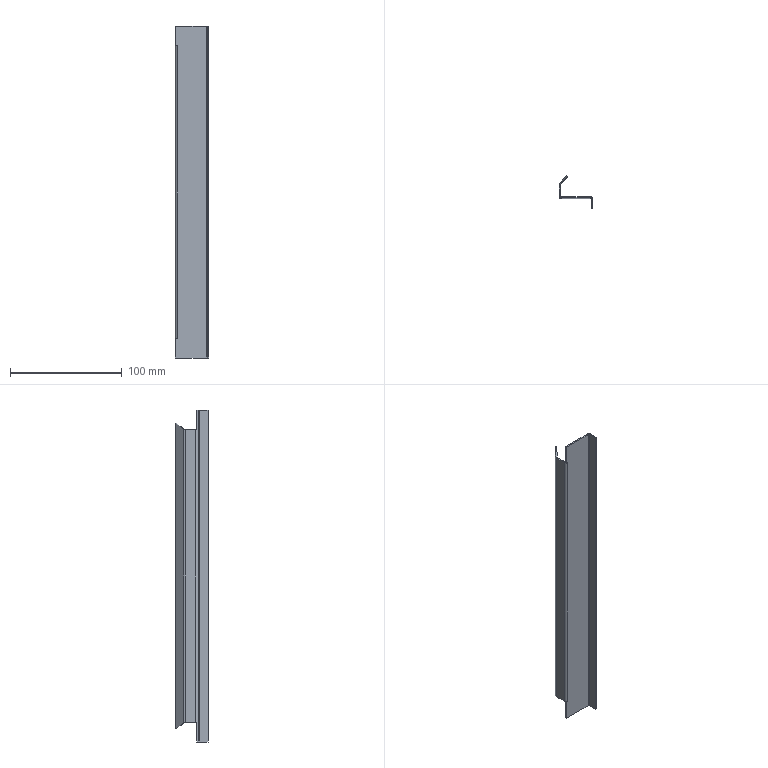Part | SolidWorks | features SMBaseFlange 2, Cut 1, FlatPattern 1, MirrorPattern 1, SheetMetal 1 | 1 solid | 38 faces | box 30.2 x 28.771 x 297.6 mm | volume 19971 mm3 | plane 30 | cylinder 6 | spline 2 | commonest cylinder face diameters 2 x3 4.4 x3
STEP:
#1=CARTESIAN_POINT('',(-28.,177.8,280.));
#2=VERTEX_POINT('',#1);
#3=CARTESIAN_POINT('',(-28.,177.8,279.8));
#4=VERTEX_POINT('',#3);
#5=CARTESIAN_POINT('',(-28.,177.8,339.311));
#6=DIRECTION('',(0.,0.,-1.));
#7=VECTOR('',#6,1000.);
#8=LINE('',#5,#7);
#9=EDGE_CURVE('',#2,#4,#8,.T.);
#10=ORIENTED_EDGE('',*,*,#9,.F.);
#11=CARTESIAN_POINT('',(-28.,179.,280.));
#12=VERTEX_POINT('',#11);
#13=CARTESIAN_POINT('',(-28.,177.8,280.));
#14=DIRECTION('',(0.,1.,0.));
#15=VECTOR('',#14,1000.);
#16=LINE('',#13,#15);
#17=EDGE_CURVE('',#2,#12,#16,.T.);
#18=ORIENTED_EDGE('',*,*,#17,.T.);
#19=CARTESIAN_POINT('',(-28.,179.,279.8));
#20=VERTEX_POINT('',#19);
#21=CARTESIAN_POINT('',(-28.,179.,339.311));
#22=DIRECTION('',(0.,0.,-1.));
#23=VECTOR('',#22,1000.);
#24=LINE('',#21,#23);
#25=EDGE_CURVE('',#12,#20,#24,.T.);
#26=ORIENTED_EDGE('',*,*,#25,.T.);
#27=CARTESIAN_POINT('',(-28.,179.,279.8));
#28=DIRECTION('',(0.,-1.,0.));
#29=VECTOR('',#28,1000.);
#30=LINE('',#27,#29);
#31=EDGE_CURVE('',#20,#4,#30,.T.);
#32=ORIENTED_EDGE('',*,*,#31,.T.);
#33=EDGE_LOOP('',(#10,#18,#26,#32));
#34=FACE_OUTER_BOUND('',#33,.T.);
#35=CARTESIAN_POINT('',(-28.,179.,288.7));
#36=DIRECTION('',(-1.,0.,0.));
#37=DIRECTION('',(0.,0.,-1.));
#38=AXIS2_PLACEMENT_3D('',#35,#36,#37);
#39=PLANE('',#38);
#40=ADVANCED_FACE('',(#34),#39,.T.);
#41=CARTESIAN_POINT('',(-29.,180.,279.8));
#42=VERTEX_POINT('',#41);
#43=CARTESIAN_POINT('',(-29.,180.,17.8));
#44=VERTEX_POINT('',#43);
#45=CARTESIAN_POINT('',(-29.,180.,339.311));
#46=DIRECTION('',(0.,0.,-1.));
#47=VECTOR('',#46,1000.);
#48=LINE('',#45,#47);
#49=EDGE_CURVE('',#42,#44,#48,.T.);
#50=ORIENTED_EDGE('',*,*,#49,.F.);
#51=CARTESIAN_POINT('',(-28.,180.,279.8));
#52=DIRECTION('',(0.,0.,1.));
#53=DIRECTION('',(0.,-1.,0.));
#54=AXIS2_PLACEMENT_3D('',#51,#52,#53);
#55=CIRCLE('',#54,1.);
#56=EDGE_CURVE('',#42,#20,#55,.T.);
#57=ORIENTED_EDGE('',*,*,#56,.T.);
#58=CARTESIAN_POINT('',(-28.,179.,17.8));
#59=VERTEX_POINT('',#58);
#60=CARTESIAN_POINT('',(-28.,179.,339.311));
#61=DIRECTION('',(0.,0.,-1.));
#62=VECTOR('',#61,1000.);
#63=LINE('',#60,#62);
#64=EDGE_CURVE('',#20,#59,#63,.T.);
#65=ORIENTED_EDGE('',*,*,#64,.T.);
#66=CARTESIAN_POINT('',(-28.,180.,17.8));
#67=DIRECTION('',(0.,0.,1.));
#68=DIRECTION('',(0.,-1.,0.));
#69=AXIS2_PLACEMENT_3D('',#66,#67,#68);
#70=CIRCLE('',#69,1.);
#71=EDGE_CURVE('',#44,#59,#70,.T.);
#72=ORIENTED_EDGE('',*,*,#71,.F.);
#73=EDGE_LOOP('',(#50,#57,#65,#72));
#74=FACE_OUTER_BOUND('',#73,.T.);
#75=CARTESIAN_POINT('',(-28.,180.,339.311));
#76=DIRECTION('',(0.,0.,-1.));
#77=DIRECTION('',(-1.,0.,0.));
#78=AXIS2_PLACEMENT_3D('',#75,#76,#77);
#79=CYLINDRICAL_SURFACE('',#78,1.);
#80=ADVANCED_FACE('',(#74),#79,.F.);
#81=CARTESIAN_POINT('',(-29.,189.636,279.8));
#82=VERTEX_POINT('',#81);
#83=CARTESIAN_POINT('',(-29.,189.636,17.8));
#84=VERTEX_POINT('',#83);
#85=CARTESIAN_POINT('',(-29.,189.636,339.311));
#86=DIRECTION('',(0.,0.,-1.));
#87=VECTOR('',#86,1000.);
#88=LINE('',#85,#87);
#89=EDGE_CURVE('',#82,#84,#88,.T.);
#90=ORIENTED_EDGE('',*,*,#89,.F.);
#91=CARTESIAN_POINT('',(-29.,190.,279.8));
#92=DIRECTION('',(0.,-1.,0.));
#93=VECTOR('',#92,1000.);
#94=LINE('',#91,#93);
#95=EDGE_CURVE('',#82,#42,#94,.T.);
#96=ORIENTED_EDGE('',*,*,#95,.T.);
#97=ORIENTED_EDGE('',*,*,#49,.T.);
#98=CARTESIAN_POINT('',(-29.,190.,17.8));
#99=DIRECTION('',(0.,-1.,0.));
#100=VECTOR('',#99,1000.);
#101=LINE('',#98,#100);
#102=EDGE_CURVE('',#84,#44,#101,.T.);
#103=ORIENTED_EDGE('',*,*,#102,.F.);
#104=EDGE_LOOP('',(#90,#96,#97,#103));
#105=FACE_OUTER_BOUND('',#104,.T.);
#106=CARTESIAN_POINT('',(-29.,190.,339.311));
#107=DIRECTION('',(1.,0.,0.));
#108=DIRECTION('',(0.,0.,-1.));
#109=AXIS2_PLACEMENT_3D('',#106,#107,#108);
#110=PLANE('',#109);
#111=ADVANCED_FACE('',(#105),#110,.T.);
#112=CARTESIAN_POINT('',(-28.766,190.279,280.034));
#113=VERTEX_POINT('',#112);
#114=CARTESIAN_POINT('',(-28.931,190.,279.8));
#115=VERTEX_POINT('',#114);
#116=CARTESIAN_POINT('',(-28.766,190.279,280.034));
#117=CARTESIAN_POINT('',(-28.836,190.195,279.964));
#118=CARTESIAN_POINT('',(-28.892,190.102,279.885));
#119=CARTESIAN_POINT('',(-28.931,190.,279.8));
#120=(BOUNDED_CURVE()B_SPLINE_CURVE(3,(#116,#117,#118,#119),.UNSPECIFIED.,.F.,.T.)B_SPLINE_CURVE_WITH_KNOTS((4,4),(4.014,4.34),.UNSPECIFIED.)CURVE()GEOMETRIC_REPRESENTATION_ITEM()RATIONAL_B_SPLINE_CURVE((1.,0.9912,0.9912,1.))REPRESENTATION_ITEM(''));
#121=EDGE_CURVE('',#113,#115,#120,.T.);
#122=ORIENTED_EDGE('',*,*,#121,.T.);
#123=CARTESIAN_POINT('',(-28.,189.636,279.8));
#124=DIRECTION('',(0.,0.,1.));
#125=DIRECTION('',(-1.,0.,0.));
#126=AXIS2_PLACEMENT_3D('',#123,#124,#125);
#127=CIRCLE('',#126,1.);
#128=EDGE_CURVE('',#115,#82,#127,.T.);
#129=ORIENTED_EDGE('',*,*,#128,.T.);
#130=ORIENTED_EDGE('',*,*,#89,.T.);
#131=CARTESIAN_POINT('',(-28.931,190.,17.8));
#132=VERTEX_POINT('',#131);
#133=CARTESIAN_POINT('',(-28.,189.636,17.8));
#134=DIRECTION('',(0.,0.,1.));
#135=DIRECTION('',(0.,-1.,0.));
#136=AXIS2_PLACEMENT_3D('',#133,#134,#135);
#137=CIRCLE('',#136,1.);
#138=EDGE_CURVE('',#132,#84,#137,.T.);
#139=ORIENTED_EDGE('',*,*,#138,.F.);
#140=CARTESIAN_POINT('',(-28.766,190.279,17.566));
#141=VERTEX_POINT('',#140);
#142=CARTESIAN_POINT('',(-28.766,190.279,17.566));
#143=CARTESIAN_POINT('',(-28.836,190.195,17.636));
#144=CARTESIAN_POINT('',(-28.892,190.102,17.715));
#145=CARTESIAN_POINT('',(-28.931,190.,17.8));
#146=(BOUNDED_CURVE()B_SPLINE_CURVE(3,(#142,#143,#144,#145),.UNSPECIFIED.,.F.,.T.)B_SPLINE_CURVE_WITH_KNOTS((4,4),(0.8727,1.198),.UNSPECIFIED.)CURVE()GEOMETRIC_REPRESENTATION_ITEM()RATIONAL_B_SPLINE_CURVE((1.,0.9912,0.9912,1.))REPRESENTATION_ITEM(''));
#147=EDGE_CURVE('',#141,#132,#146,.T.);
#148=ORIENTED_EDGE('',*,*,#147,.F.);
#149=CARTESIAN_POINT('',(-28.766,190.279,339.311));
#150=DIRECTION('',(0.,0.,-1.));
#151=VECTOR('',#150,1000.);
#152=LINE('',#149,#151);
#153=EDGE_CURVE('',#113,#141,#152,.T.);
#154=ORIENTED_EDGE('',*,*,#153,.F.);
#155=EDGE_LOOP('',(#122,#129,#130,#139,#148,#154));
#156=FACE_OUTER_BOUND('',#155,.T.);
#157=CARTESIAN_POINT('',(-28.,189.636,339.311));
#158=DIRECTION('',(0.,0.,-1.));
#159=DIRECTION('',(-1.,0.,0.));
#160=AXIS2_PLACEMENT_3D('',#157,#158,#159);
#161=CYLINDRICAL_SURFACE('',#160,1.);
#162=ADVANCED_FACE('',(#156),#161,.F.);
#163=CARTESIAN_POINT('',(-23.126,197.,285.674));
#164=VERTEX_POINT('',#163);
#165=CARTESIAN_POINT('',(-23.126,197.,11.926));
#166=VERTEX_POINT('',#165);
#167=CARTESIAN_POINT('',(-23.126,197.,339.311));
#168=DIRECTION('',(0.,0.,-1.));
#169=VECTOR('',#168,1000.);
#170=LINE('',#167,#169);
#171=EDGE_CURVE('',#164,#166,#170,.T.);
#172=ORIENTED_EDGE('',*,*,#171,.F.);
#173=CARTESIAN_POINT('',(-7.444,215.689,301.356));
#174=DIRECTION('',(-0.5407,-0.6444,-0.5407));
#175=VECTOR('',#174,1000.);
#176=LINE('',#173,#175);
#177=EDGE_CURVE('',#164,#113,#176,.T.);
#178=ORIENTED_EDGE('',*,*,#177,.T.);
#179=ORIENTED_EDGE('',*,*,#153,.T.);
#180=CARTESIAN_POINT('',(-118.845,82.927,107.645));
#181=DIRECTION('',(-0.5407,-0.6444,0.5407));
#182=VECTOR('',#181,1000.);
#183=LINE('',#180,#182);
#184=EDGE_CURVE('',#166,#141,#183,.T.);
#185=ORIENTED_EDGE('',*,*,#184,.F.);
#186=EDGE_LOOP('',(#172,#178,#179,#185));
#187=FACE_OUTER_BOUND('',#186,.T.);
#188=CARTESIAN_POINT('',(-23.126,197.,339.311));
#189=DIRECTION('',(0.766,-0.6428,0.));
#190=DIRECTION('',(0.6428,0.766,0.));
#191=AXIS2_PLACEMENT_3D('',#188,#189,#190);
#192=PLANE('',#191);
#193=ADVANCED_FACE('',(#187),#192,.T.);
#194=CARTESIAN_POINT('',(-24.046,197.771,285.674));
#195=VERTEX_POINT('',#194);
#196=CARTESIAN_POINT('',(-24.046,197.771,11.926));
#197=VERTEX_POINT('',#196);
#198=CARTESIAN_POINT('',(-24.046,197.771,339.311));
#199=DIRECTION('',(0.,0.,-1.));
#200=VECTOR('',#199,1000.);
#201=LINE('',#198,#200);
#202=EDGE_CURVE('',#195,#197,#201,.T.);
#203=ORIENTED_EDGE('',*,*,#202,.F.);
#204=CARTESIAN_POINT('',(-23.126,197.,285.674));
#205=DIRECTION('',(-0.766,0.6428,0.));
#206=VECTOR('',#205,1000.);
#207=LINE('',#204,#206);
#208=EDGE_CURVE('',#164,#195,#207,.T.);
#209=ORIENTED_EDGE('',*,*,#208,.F.);
#210=ORIENTED_EDGE('',*,*,#171,.T.);
#211=CARTESIAN_POINT('',(-23.126,197.,11.926));
#212=DIRECTION('',(-0.766,0.6428,0.));
#213=VECTOR('',#212,1000.);
#214=LINE('',#211,#213);
#215=EDGE_CURVE('',#166,#197,#214,.T.);
#216=ORIENTED_EDGE('',*,*,#215,.T.);
#217=EDGE_LOOP('',(#203,#209,#210,#216));
#218=FACE_OUTER_BOUND('',#217,.T.);
#219=CARTESIAN_POINT('',(-24.046,197.771,339.311));
#220=DIRECTION('',(0.6428,0.766,0.));
#221=DIRECTION('',(-0.766,0.6428,0.));
#222=AXIS2_PLACEMENT_3D('',#219,#220,#221);
#223=PLANE('',#222);
#224=ADVANCED_FACE('',(#218),#223,.T.);
#225=CARTESIAN_POINT('',(-29.685,191.05,280.034));
#226=VERTEX_POINT('',#225);
#227=CARTESIAN_POINT('',(-8.363,216.461,301.356));
#228=DIRECTION('',(-0.5407,-0.6444,-0.5407));
#229=VECTOR('',#228,1000.);
#230=LINE('',#227,#229);
#231=EDGE_CURVE('',#195,#226,#230,.T.);
#232=ORIENTED_EDGE('',*,*,#231,.F.);
#233=ORIENTED_EDGE('',*,*,#202,.T.);
#234=CARTESIAN_POINT('',(-29.685,191.05,17.566));
#235=VERTEX_POINT('',#234);
#236=CARTESIAN_POINT('',(-119.764,83.698,107.645));
#237=DIRECTION('',(-0.5407,-0.6444,0.5407));
#238=VECTOR('',#237,1000.);
#239=LINE('',#236,#238);
#240=EDGE_CURVE('',#197,#235,#239,.T.);
#241=ORIENTED_EDGE('',*,*,#240,.T.);
#242=CARTESIAN_POINT('',(-29.685,191.05,339.311));
#243=DIRECTION('',(0.,0.,-1.));
#244=VECTOR('',#243,1000.);
#245=LINE('',#242,#244);
#246=EDGE_CURVE('',#226,#235,#245,.T.);
#247=ORIENTED_EDGE('',*,*,#246,.F.);
#248=EDGE_LOOP('',(#232,#233,#241,#247));
#249=FACE_OUTER_BOUND('',#248,.T.);
#250=CARTESIAN_POINT('',(-24.046,197.771,339.311));
#251=DIRECTION('',(0.766,-0.6428,0.));
#252=DIRECTION('',(0.6428,0.766,0.));
#253=AXIS2_PLACEMENT_3D('',#250,#251,#252);
#254=PLANE('',#253);
#255=ADVANCED_FACE('',(#249),#254,.F.);
#256=CARTESIAN_POINT('',(-30.049,190.437,279.8));
#257=VERTEX_POINT('',#256);
#258=CARTESIAN_POINT('',(-30.2,189.636,279.8));
#259=VERTEX_POINT('',#258);
#260=CARTESIAN_POINT('',(-28.,189.636,279.8));
#261=DIRECTION('',(0.,0.,1.));
#262=DIRECTION('',(0.,-1.,0.));
#263=AXIS2_PLACEMENT_3D('',#260,#261,#262);
#264=CIRCLE('',#263,2.2);
#265=EDGE_CURVE('',#257,#259,#264,.T.);
#266=ORIENTED_EDGE('',*,*,#265,.F.);
#267=CARTESIAN_POINT('',(-29.685,191.05,280.034));
#268=CARTESIAN_POINT('',(-29.839,190.866,279.964));
#269=CARTESIAN_POINT('',(-29.962,190.66,279.885));
#270=CARTESIAN_POINT('',(-30.049,190.437,279.8));
#271=(BOUNDED_CURVE()B_SPLINE_CURVE(3,(#267,#268,#269,#270),.UNSPECIFIED.,.F.,.T.)B_SPLINE_CURVE_WITH_KNOTS((4,4),(4.014,4.34),.UNSPECIFIED.)CURVE()GEOMETRIC_REPRESENTATION_ITEM()RATIONAL_B_SPLINE_CURVE((1.,0.9912,0.9912,1.))REPRESENTATION_ITEM(''));
#272=EDGE_CURVE('',#226,#257,#271,.T.);
#273=ORIENTED_EDGE('',*,*,#272,.F.);
#274=ORIENTED_EDGE('',*,*,#246,.T.);
#275=CARTESIAN_POINT('',(-30.049,190.437,17.8));
#276=VERTEX_POINT('',#275);
#277=CARTESIAN_POINT('',(-29.685,191.05,17.566));
#278=CARTESIAN_POINT('',(-29.839,190.866,17.636));
#279=CARTESIAN_POINT('',(-29.962,190.66,17.715));
#280=CARTESIAN_POINT('',(-30.049,190.437,17.8));
#281=(BOUNDED_CURVE()B_SPLINE_CURVE(3,(#277,#278,#279,#280),.UNSPECIFIED.,.F.,.T.)B_SPLINE_CURVE_WITH_KNOTS((4,4),(0.8727,1.198),.UNSPECIFIED.)CURVE()GEOMETRIC_REPRESENTATION_ITEM()RATIONAL_B_SPLINE_CURVE((1.,0.9912,0.9912,1.))REPRESENTATION_ITEM(''));
#282=EDGE_CURVE('',#235,#276,#281,.T.);
#283=ORIENTED_EDGE('',*,*,#282,.T.);
#284=CARTESIAN_POINT('',(-30.2,189.636,17.8));
#285=VERTEX_POINT('',#284);
#286=CARTESIAN_POINT('',(-28.,189.636,17.8));
#287=DIRECTION('',(0.,0.,1.));
#288=DIRECTION('',(-1.,0.,0.));
#289=AXIS2_PLACEMENT_3D('',#286,#287,#288);
#290=CIRCLE('',#289,2.2);
#291=EDGE_CURVE('',#276,#285,#290,.T.);
#292=ORIENTED_EDGE('',*,*,#291,.T.);
#293=CARTESIAN_POINT('',(-30.2,189.636,339.311));
#294=DIRECTION('',(0.,0.,-1.));
#295=VECTOR('',#294,1000.);
#296=LINE('',#293,#295);
#297=EDGE_CURVE('',#259,#285,#296,.T.);
#298=ORIENTED_EDGE('',*,*,#297,.F.);
#299=EDGE_LOOP('',(#266,#273,#274,#283,#292,#298));
#300=FACE_OUTER_BOUND('',#299,.T.);
#301=CARTESIAN_POINT('',(-28.,189.636,339.311));
#302=DIRECTION('',(0.,0.,-1.));
#303=DIRECTION('',(-1.,0.,0.));
#304=AXIS2_PLACEMENT_3D('',#301,#302,#303);
#305=CYLINDRICAL_SURFACE('',#304,2.2);
#306=ADVANCED_FACE('',(#300),#305,.T.);
#307=CARTESIAN_POINT('',(-30.2,180.,279.8));
#308=VERTEX_POINT('',#307);
#309=CARTESIAN_POINT('',(-30.2,190.,279.8));
#310=DIRECTION('',(0.,-1.,0.));
#311=VECTOR('',#310,1000.);
#312=LINE('',#309,#311);
#313=EDGE_CURVE('',#259,#308,#312,.T.);
#314=ORIENTED_EDGE('',*,*,#313,.F.);
#315=ORIENTED_EDGE('',*,*,#297,.T.);
#316=CARTESIAN_POINT('',(-30.2,180.,17.8));
#317=VERTEX_POINT('',#316);
#318=CARTESIAN_POINT('',(-30.2,190.,17.8));
#319=DIRECTION('',(0.,-1.,0.));
#320=VECTOR('',#319,1000.);
#321=LINE('',#318,#320);
#322=EDGE_CURVE('',#285,#317,#321,.T.);
#323=ORIENTED_EDGE('',*,*,#322,.T.);
#324=CARTESIAN_POINT('',(-30.2,180.,339.311));
#325=DIRECTION('',(0.,0.,-1.));
#326=VECTOR('',#325,1000.);
#327=LINE('',#324,#326);
#328=EDGE_CURVE('',#308,#317,#327,.T.);
#329=ORIENTED_EDGE('',*,*,#328,.F.);
#330=EDGE_LOOP('',(#314,#315,#323,#329));
#331=FACE_OUTER_BOUND('',#330,.T.);
#332=CARTESIAN_POINT('',(-30.2,190.,339.311));
#333=DIRECTION('',(1.,0.,0.));
#334=DIRECTION('',(0.,0.,-1.));
#335=AXIS2_PLACEMENT_3D('',#332,#333,#334);
#336=PLANE('',#335);
#337=ADVANCED_FACE('',(#331),#336,.F.);
#338=CARTESIAN_POINT('',(-28.,180.,279.8));
#339=DIRECTION('',(0.,0.,1.));
#340=DIRECTION('',(-1.,0.,0.));
#341=AXIS2_PLACEMENT_3D('',#338,#339,#340);
#342=CIRCLE('',#341,2.2);
#343=EDGE_CURVE('',#308,#4,#342,.T.);
#344=ORIENTED_EDGE('',*,*,#343,.F.);
#345=ORIENTED_EDGE('',*,*,#328,.T.);
#346=CARTESIAN_POINT('',(-28.,177.8,17.8));
#347=VERTEX_POINT('',#346);
#348=CARTESIAN_POINT('',(-28.,180.,17.8));
#349=DIRECTION('',(0.,0.,1.));
#350=DIRECTION('',(-1.,0.,0.));
#351=AXIS2_PLACEMENT_3D('',#348,#349,#350);
#352=CIRCLE('',#351,2.2);
#353=EDGE_CURVE('',#317,#347,#352,.T.);
#354=ORIENTED_EDGE('',*,*,#353,.T.);
#355=CARTESIAN_POINT('',(-28.,177.8,339.311));
#356=DIRECTION('',(0.,0.,-1.));
#357=VECTOR('',#356,1000.);
#358=LINE('',#355,#357);
#359=EDGE_CURVE('',#4,#347,#358,.T.);
#360=ORIENTED_EDGE('',*,*,#359,.F.);
#361=EDGE_LOOP('',(#344,#345,#354,#360));
#362=FACE_OUTER_BOUND('',#361,.T.);
#363=CARTESIAN_POINT('',(-28.,180.,339.311));
#364=DIRECTION('',(0.,0.,-1.));
#365=DIRECTION('',(-1.,0.,0.));
#366=AXIS2_PLACEMENT_3D('',#363,#364,#365);
#367=CYLINDRICAL_SURFACE('',#366,2.2);
#368=ADVANCED_FACE('',(#362),#367,.T.);
#369=CARTESIAN_POINT('',(-2.2,179.,0.));
#370=VERTEX_POINT('',#369);
#371=CARTESIAN_POINT('',(-2.2,177.8,0.));
#372=VERTEX_POINT('',#371);
#373=CARTESIAN_POINT('',(-2.2,179.,0.));
#374=DIRECTION('',(0.,-1.,0.));
#375=VECTOR('',#374,1000.);
#376=LINE('',#373,#375);
#377=EDGE_CURVE('',#370,#372,#376,.T.);
#378=ORIENTED_EDGE('',*,*,#377,.F.);
#379=CARTESIAN_POINT('',(0.,176.8,0.));
#380=VERTEX_POINT('',#379);
#381=CARTESIAN_POINT('',(-2.2,176.8,0.));
#382=DIRECTION('',(0.,0.,-1.));
#383=DIRECTION('',(1.,0.,0.));
#384=AXIS2_PLACEMENT_3D('',#381,#382,#383);
#385=CIRCLE('',#384,2.2);
#386=EDGE_CURVE('',#370,#380,#385,.T.);
#387=ORIENTED_EDGE('',*,*,#386,.T.);
#388=CARTESIAN_POINT('',(-1.2,176.8,0.));
#389=VERTEX_POINT('',#388);
#390=CARTESIAN_POINT('',(-1.2,176.8,0.));
#391=DIRECTION('',(1.,0.,0.));
#392=VECTOR('',#391,1000.);
#393=LINE('',#390,#392);
#394=EDGE_CURVE('',#389,#380,#393,.T.);
#395=ORIENTED_EDGE('',*,*,#394,.F.);
#396=CARTESIAN_POINT('',(-2.2,176.8,0.));
#397=DIRECTION('',(0.,0.,-1.));
#398=DIRECTION('',(1.,0.,0.));
#399=AXIS2_PLACEMENT_3D('',#396,#397,#398);
#400=CIRCLE('',#399,1.);
#401=EDGE_CURVE('',#372,#389,#400,.T.);
#402=ORIENTED_EDGE('',*,*,#401,.F.);
#403=EDGE_LOOP('',(#378,#387,#395,#402));
#404=FACE_OUTER_BOUND('',#403,.T.);
#405=CARTESIAN_POINT('',(-2.2,179.,0.));
#406=DIRECTION('',(0.,0.,-1.));
#407=DIRECTION('',(-1.,0.,0.));
#408=AXIS2_PLACEMENT_3D('',#405,#406,#407);
#409=PLANE('',#408);
#410=ADVANCED_FACE('',(#404),#409,.T.);
#411=CARTESIAN_POINT('',(-29.9,179.,0.));
#412=VERTEX_POINT('',#411);
#413=CARTESIAN_POINT('',(-29.,179.,0.));
#414=DIRECTION('',(1.,0.,0.));
#415=VECTOR('',#414,1000.);
#416=LINE('',#413,#415);
#417=EDGE_CURVE('',#412,#370,#416,.T.);
#418=ORIENTED_EDGE('',*,*,#417,.T.);
#419=ORIENTED_EDGE('',*,*,#377,.T.);
#420=CARTESIAN_POINT('',(-29.9,177.8,0.));
#421=VERTEX_POINT('',#420);
#422=CARTESIAN_POINT('',(-29.,177.8,0.));
#423=DIRECTION('',(1.,0.,0.));
#424=VECTOR('',#423,1000.);
#425=LINE('',#422,#424);
#426=EDGE_CURVE('',#421,#372,#425,.T.);
#427=ORIENTED_EDGE('',*,*,#426,.F.);
#428=CARTESIAN_POINT('',(-29.9,177.8,0.));
#429=DIRECTION('',(0.,1.,0.));
#430=VECTOR('',#429,1000.);
#431=LINE('',#428,#430);
#432=EDGE_CURVE('',#421,#412,#431,.T.);
#433=ORIENTED_EDGE('',*,*,#432,.T.);
#434=EDGE_LOOP('',(#418,#419,#427,#433));
#435=FACE_OUTER_BOUND('',#434,.T.);
#436=CARTESIAN_POINT('',(-1.2,176.8,0.));
#437=DIRECTION('',(0.,0.,-1.));
#438=DIRECTION('',(-1.,0.,0.));
#439=AXIS2_PLACEMENT_3D('',#436,#437,#438);
#440=PLANE('',#439);
#441=ADVANCED_FACE('',(#435),#440,.T.);
#442=CARTESIAN_POINT('',(-1.2,176.8,297.6));
#443=VERTEX_POINT('',#442);
#444=CARTESIAN_POINT('',(-1.2,169.,297.6));
#445=VERTEX_POINT('',#444);
#446=CARTESIAN_POINT('',(-1.2,179.,297.6));
#447=DIRECTION('',(0.,-1.,0.));
#448=VECTOR('',#447,1000.);
#449=LINE('',#446,#448);
#450=EDGE_CURVE('',#443,#445,#449,.T.);
#451=ORIENTED_EDGE('',*,*,#450,.F.);
#452=CARTESIAN_POINT('',(-1.2,176.8,339.311));
#453=DIRECTION('',(0.,0.,-1.));
#454=VECTOR('',#453,1000.);
#455=LINE('',#452,#454);
#456=EDGE_CURVE('',#443,#389,#455,.T.);
#457=ORIENTED_EDGE('',*,*,#456,.T.);
#458=CARTESIAN_POINT('',(-1.2,169.,0.));
#459=VERTEX_POINT('',#458);
#460=CARTESIAN_POINT('',(-1.2,179.,0.));
#461=DIRECTION('',(0.,-1.,0.));
#462=VECTOR('',#461,1000.);
#463=LINE('',#460,#462);
#464=EDGE_CURVE('',#389,#459,#463,.T.);
#465=ORIENTED_EDGE('',*,*,#464,.T.);
#466=CARTESIAN_POINT('',(-1.2,169.,339.311));
#467=DIRECTION('',(0.,0.,-1.));
#468=VECTOR('',#467,1000.);
#469=LINE('',#466,#468);
#470=EDGE_CURVE('',#445,#459,#469,.T.);
#471=ORIENTED_EDGE('',*,*,#470,.F.);
#472=EDGE_LOOP('',(#451,#457,#465,#471));
#473=FACE_OUTER_BOUND('',#472,.T.);
#474=CARTESIAN_POINT('',(-1.2,179.,339.311));
#475=DIRECTION('',(1.,0.,0.));
#476=DIRECTION('',(0.,1.,0.));
#477=AXIS2_PLACEMENT_3D('',#474,#475,#476);
#478=PLANE('',#477);
#479=ADVANCED_FACE('',(#473),#478,.F.);
#480=CARTESIAN_POINT('',(0.,169.,297.6));
#481=VERTEX_POINT('',#480);
#482=CARTESIAN_POINT('',(0.,169.,0.));
#483=VERTEX_POINT('',#482);
#484=CARTESIAN_POINT('',(0.,169.,339.311));
#485=DIRECTION('',(0.,0.,-1.));
#486=VECTOR('',#485,1000.);
#487=LINE('',#484,#486);
#488=EDGE_CURVE('',#481,#483,#487,.T.);
#489=ORIENTED_EDGE('',*,*,#488,.F.);
#490=CARTESIAN_POINT('',(0.,169.,297.6));
#491=DIRECTION('',(-1.,0.,0.));
#492=VECTOR('',#491,1000.);
#493=LINE('',#490,#492);
#494=EDGE_CURVE('',#481,#445,#493,.T.);
#495=ORIENTED_EDGE('',*,*,#494,.T.);
#496=ORIENTED_EDGE('',*,*,#470,.T.);
#497=CARTESIAN_POINT('',(0.,169.,0.));
#498=DIRECTION('',(-1.,0.,0.));
#499=VECTOR('',#498,1000.);
#500=LINE('',#497,#499);
#501=EDGE_CURVE('',#483,#459,#500,.T.);
#502=ORIENTED_EDGE('',*,*,#501,.F.);
#503=EDGE_LOOP('',(#489,#495,#496,#502));
#504=FACE_OUTER_BOUND('',#503,.T.);
#505=CARTESIAN_POINT('',(0.,169.,339.311));
#506=DIRECTION('',(0.,-1.,0.));
#507=DIRECTION('',(0.,0.,-1.));
#508=AXIS2_PLACEMENT_3D('',#505,#506,#507);
#509=PLANE('',#508);
#510=ADVANCED_FACE('',(#504),#509,.T.);
#511=CARTESIAN_POINT('',(0.,176.8,297.6));
#512=VERTEX_POINT('',#511);
#513=CARTESIAN_POINT('',(0.,176.8,339.311));
#514=DIRECTION('',(0.,0.,-1.));
#515=VECTOR('',#514,1000.);
#516=LINE('',#513,#515);
#517=EDGE_CURVE('',#512,#380,#516,.T.);
#518=ORIENTED_EDGE('',*,*,#517,.F.);
#519=CARTESIAN_POINT('',(0.,179.,297.6));
#520=DIRECTION('',(0.,-1.,0.));
#521=VECTOR('',#520,1000.);
#522=LINE('',#519,#521);
#523=EDGE_CURVE('',#512,#481,#522,.T.);
#524=ORIENTED_EDGE('',*,*,#523,.T.);
#525=ORIENTED_EDGE('',*,*,#488,.T.);
#526=CARTESIAN_POINT('',(0.,179.,0.));
#527=DIRECTION('',(0.,-1.,0.));
#528=VECTOR('',#527,1000.);
#529=LINE('',#526,#528);
#530=EDGE_CURVE('',#380,#483,#529,.T.);
#531=ORIENTED_EDGE('',*,*,#530,.F.);
#532=EDGE_LOOP('',(#518,#524,#525,#531));
#533=FACE_OUTER_BOUND('',#532,.T.);
#534=CARTESIAN_POINT('',(0.,179.,339.311));
#535=DIRECTION('',(1.,0.,0.));
#536=DIRECTION('',(0.,1.,0.));
#537=AXIS2_PLACEMENT_3D('',#534,#535,#536);
#538=PLANE('',#537);
#539=ADVANCED_FACE('',(#533),#538,.T.);
#540=CARTESIAN_POINT('',(-2.2,179.,297.6));
#541=VERTEX_POINT('',#540);
#542=CARTESIAN_POINT('',(-2.2,179.,339.311));
#543=DIRECTION('',(0.,0.,-1.));
#544=VECTOR('',#543,1000.);
#545=LINE('',#542,#544);
#546=EDGE_CURVE('',#541,#370,#545,.T.);
#547=ORIENTED_EDGE('',*,*,#546,.F.);
#548=CARTESIAN_POINT('',(-2.2,176.8,297.6));
#549=DIRECTION('',(0.,0.,-1.));
#550=DIRECTION('',(-1.,0.,0.));
#551=AXIS2_PLACEMENT_3D('',#548,#549,#550);
#552=CIRCLE('',#551,2.2);
#553=EDGE_CURVE('',#541,#512,#552,.T.);
#554=ORIENTED_EDGE('',*,*,#553,.T.);
#555=ORIENTED_EDGE('',*,*,#517,.T.);
#556=ORIENTED_EDGE('',*,*,#386,.F.);
#557=EDGE_LOOP('',(#547,#554,#555,#556));
#558=FACE_OUTER_BOUND('',#557,.T.);
#559=CARTESIAN_POINT('',(-2.2,176.8,339.311));
#560=DIRECTION('',(0.,0.,-1.));
#561=DIRECTION('',(-1.,0.,0.));
#562=AXIS2_PLACEMENT_3D('',#559,#560,#561);
#563=CYLINDRICAL_SURFACE('',#562,2.2);
#564=ADVANCED_FACE('',(#558),#563,.T.);
#565=ORIENTED_EDGE('',*,*,#25,.F.);
#566=CARTESIAN_POINT('',(-29.9,179.,280.));
#567=VERTEX_POINT('',#566);
#568=CARTESIAN_POINT('',(-28.,179.,280.));
#569=DIRECTION('',(1.,0.,0.));
#570=VECTOR('',#569,1000.);
#571=LINE('',#568,#570);
#572=EDGE_CURVE('',#567,#12,#571,.T.);
#573=ORIENTED_EDGE('',*,*,#572,.F.);
#574=CARTESIAN_POINT('',(-29.9,179.,297.6));
#575=VERTEX_POINT('',#574);
#576=CARTESIAN_POINT('',(-29.9,179.,297.6));
#577=DIRECTION('',(0.,0.,-1.));
#578=VECTOR('',#577,1000.);
#579=LINE('',#576,#578);
#580=EDGE_CURVE('',#575,#567,#579,.T.);
#581=ORIENTED_EDGE('',*,*,#580,.F.);
#582=CARTESIAN_POINT('',(-29.,179.,297.6));
#583=DIRECTION('',(1.,0.,0.));
#584=VECTOR('',#583,1000.);
#585=LINE('',#582,#584);
#586=EDGE_CURVE('',#575,#541,#585,.T.);
#587=ORIENTED_EDGE('',*,*,#586,.T.);
#588=ORIENTED_EDGE('',*,*,#546,.T.);
#589=ORIENTED_EDGE('',*,*,#417,.F.);
#590=CARTESIAN_POINT('',(-29.9,179.,17.6));
#591=VERTEX_POINT('',#590);
#592=CARTESIAN_POINT('',(-29.9,179.,0.));
#593=DIRECTION('',(0.,0.,1.));
#594=VECTOR('',#593,1000.);
#595=LINE('',#592,#594);
#596=EDGE_CURVE('',#412,#591,#595,.T.);
#597=ORIENTED_EDGE('',*,*,#596,.T.);
#598=CARTESIAN_POINT('',(-28.,179.,17.6));
#599=VERTEX_POINT('',#598);
#600=CARTESIAN_POINT('',(-28.,179.,17.6));
#601=DIRECTION('',(1.,0.,0.));
#602=VECTOR('',#601,1000.);
#603=LINE('',#600,#602);
#604=EDGE_CURVE('',#591,#599,#603,.T.);
#605=ORIENTED_EDGE('',*,*,#604,.T.);
#606=CARTESIAN_POINT('',(-28.,179.,339.311));
#607=DIRECTION('',(0.,0.,-1.));
#608=VECTOR('',#607,1000.);
#609=LINE('',#606,#608);
#610=EDGE_CURVE('',#59,#599,#609,.T.);
#611=ORIENTED_EDGE('',*,*,#610,.F.);
#612=ORIENTED_EDGE('',*,*,#64,.F.);
#613=EDGE_LOOP('',(#565,#573,#581,#587,#588,#589,#597,#605,#611,#612));
#614=FACE_OUTER_BOUND('',#613,.T.);
#615=CARTESIAN_POINT('',(-29.,179.,339.311));
#616=DIRECTION('',(0.,1.,0.));
#617=DIRECTION('',(0.,0.,1.));
#618=AXIS2_PLACEMENT_3D('',#615,#616,#617);
#619=PLANE('',#618);
#620=ADVANCED_FACE('',(#614),#619,.T.);
#621=CARTESIAN_POINT('',(-29.9,177.8,297.6));
#622=VERTEX_POINT('',#621);
#623=CARTESIAN_POINT('',(-2.2,177.8,297.6));
#624=VERTEX_POINT('',#623);
#625=CARTESIAN_POINT('',(-29.,177.8,297.6));
#626=DIRECTION('',(1.,0.,0.));
#627=VECTOR('',#626,1000.);
#628=LINE('',#625,#627);
#629=EDGE_CURVE('',#622,#624,#628,.T.);
#630=ORIENTED_EDGE('',*,*,#629,.F.);
#631=CARTESIAN_POINT('',(-29.9,177.8,280.));
#632=VERTEX_POINT('',#631);
#633=CARTESIAN_POINT('',(-29.9,177.8,297.6));
#634=DIRECTION('',(0.,0.,-1.));
#635=VECTOR('',#634,1000.);
#636=LINE('',#633,#635);
#637=EDGE_CURVE('',#622,#632,#636,.T.);
#638=ORIENTED_EDGE('',*,*,#637,.T.);
#639=CARTESIAN_POINT('',(-28.,177.8,280.));
#640=DIRECTION('',(1.,0.,0.));
#641=VECTOR('',#640,1000.);
#642=LINE('',#639,#641);
#643=EDGE_CURVE('',#632,#2,#642,.T.);
#644=ORIENTED_EDGE('',*,*,#643,.T.);
#645=ORIENTED_EDGE('',*,*,#9,.T.);
#646=ORIENTED_EDGE('',*,*,#359,.T.);
#647=CARTESIAN_POINT('',(-28.,177.8,17.6));
#648=VERTEX_POINT('',#647);
#649=CARTESIAN_POINT('',(-28.,177.8,339.311));
#650=DIRECTION('',(0.,0.,-1.));
#651=VECTOR('',#650,1000.);
#652=LINE('',#649,#651);
#653=EDGE_CURVE('',#347,#648,#652,.T.);
#654=ORIENTED_EDGE('',*,*,#653,.T.);
#655=CARTESIAN_POINT('',(-29.9,177.8,17.6));
#656=VERTEX_POINT('',#655);
#657=CARTESIAN_POINT('',(-28.,177.8,17.6));
#658=DIRECTION('',(1.,0.,0.));
#659=VECTOR('',#658,1000.);
#660=LINE('',#657,#659);
#661=EDGE_CURVE('',#656,#648,#660,.T.);
#662=ORIENTED_EDGE('',*,*,#661,.F.);
#663=CARTESIAN_POINT('',(-29.9,177.8,0.));
#664=DIRECTION('',(0.,0.,1.));
#665=VECTOR('',#664,1000.);
#666=LINE('',#663,#665);
#667=EDGE_CURVE('',#421,#656,#666,.T.);
#668=ORIENTED_EDGE('',*,*,#667,.F.);
#669=ORIENTED_EDGE('',*,*,#426,.T.);
#670=CARTESIAN_POINT('',(-2.2,177.8,339.311));
#671=DIRECTION('',(0.,0.,-1.));
#672=VECTOR('',#671,1000.);
#673=LINE('',#670,#672);
#674=EDGE_CURVE('',#624,#372,#673,.T.);
#675=ORIENTED_EDGE('',*,*,#674,.F.);
#676=EDGE_LOOP('',(#630,#638,#644,#645,#646,#654,#662,#668,#669,#675));
#677=FACE_OUTER_BOUND('',#676,.T.);
#678=CARTESIAN_POINT('',(-29.,177.8,339.311));
#679=DIRECTION('',(0.,1.,0.));
#680=DIRECTION('',(0.,0.,1.));
#681=AXIS2_PLACEMENT_3D('',#678,#679,#680);
#682=PLANE('',#681);
#683=ADVANCED_FACE('',(#677),#682,.F.);
#684=CARTESIAN_POINT('',(-2.2,176.8,297.6));
#685=DIRECTION('',(0.,0.,-1.));
#686=DIRECTION('',(0.,-1.,0.));
#687=AXIS2_PLACEMENT_3D('',#684,#685,#686);
#688=CIRCLE('',#687,1.);
#689=EDGE_CURVE('',#624,#443,#688,.T.);
#690=ORIENTED_EDGE('',*,*,#689,.F.);
#691=ORIENTED_EDGE('',*,*,#674,.T.);
#692=ORIENTED_EDGE('',*,*,#401,.T.);
#693=ORIENTED_EDGE('',*,*,#456,.F.);
#694=EDGE_LOOP('',(#690,#691,#692,#693));
#695=FACE_OUTER_BOUND('',#694,.T.);
#696=CARTESIAN_POINT('',(-2.2,176.8,339.311));
#697=DIRECTION('',(0.,0.,-1.));
#698=DIRECTION('',(-1.,0.,0.));
#699=AXIS2_PLACEMENT_3D('',#696,#697,#698);
#700=CYLINDRICAL_SURFACE('',#699,1.);
#701=ADVANCED_FACE('',(#695),#700,.F.);
#702=ORIENTED_EDGE('',*,*,#464,.F.);
#703=ORIENTED_EDGE('',*,*,#394,.T.);
#704=ORIENTED_EDGE('',*,*,#530,.T.);
#705=ORIENTED_EDGE('',*,*,#501,.T.);
#706=EDGE_LOOP('',(#702,#703,#704,#705));
#707=FACE_OUTER_BOUND('',#706,.T.);
#708=CARTESIAN_POINT('',(-2.2,176.8,0.));
#709=DIRECTION('',(0.,0.,1.));
#710=DIRECTION('',(1.,0.,0.));
#711=AXIS2_PLACEMENT_3D('',#708,#709,#710);
#712=PLANE('',#711);
#713=ADVANCED_FACE('',(#707),#712,.F.);
#714=ORIENTED_EDGE('',*,*,#629,.T.);
#715=CARTESIAN_POINT('',(-2.2,177.8,297.6));
#716=DIRECTION('',(0.,1.,0.));
#717=VECTOR('',#716,1000.);
#718=LINE('',#715,#717);
#719=EDGE_CURVE('',#624,#541,#718,.T.);
#720=ORIENTED_EDGE('',*,*,#719,.T.);
#721=ORIENTED_EDGE('',*,*,#586,.F.);
#722=CARTESIAN_POINT('',(-29.9,177.8,297.6));
#723=DIRECTION('',(0.,1.,0.));
#724=VECTOR('',#723,1000.);
#725=LINE('',#722,#724);
#726=EDGE_CURVE('',#622,#575,#725,.T.);
#727=ORIENTED_EDGE('',*,*,#726,.F.);
#728=EDGE_LOOP('',(#714,#720,#721,#727));
#729=FACE_OUTER_BOUND('',#728,.T.);
#730=CARTESIAN_POINT('',(-29.,177.8,297.6));
#731=DIRECTION('',(0.,0.,1.));
#732=DIRECTION('',(1.,0.,0.));
#733=AXIS2_PLACEMENT_3D('',#730,#731,#732);
#734=PLANE('',#733);
#735=ADVANCED_FACE('',(#729),#734,.T.);
#736=ORIENTED_EDGE('',*,*,#494,.F.);
#737=ORIENTED_EDGE('',*,*,#523,.F.);
#738=CARTESIAN_POINT('',(0.,176.8,297.6));
#739=DIRECTION('',(-1.,0.,0.));
#740=VECTOR('',#739,1000.);
#741=LINE('',#738,#740);
#742=EDGE_CURVE('',#512,#443,#741,.T.);
#743=ORIENTED_EDGE('',*,*,#742,.T.);
#744=ORIENTED_EDGE('',*,*,#450,.T.);
#745=EDGE_LOOP('',(#736,#737,#743,#744));
#746=FACE_OUTER_BOUND('',#745,.T.);
#747=CARTESIAN_POINT('',(0.,179.,297.6));
#748=DIRECTION('',(0.,0.,1.));
#749=DIRECTION('',(0.,-1.,0.));
#750=AXIS2_PLACEMENT_3D('',#747,#748,#749);
#751=PLANE('',#750);
#752=ADVANCED_FACE('',(#746),#751,.T.);
#753=ORIENTED_EDGE('',*,*,#689,.T.);
#754=ORIENTED_EDGE('',*,*,#742,.F.);
#755=ORIENTED_EDGE('',*,*,#553,.F.);
#756=ORIENTED_EDGE('',*,*,#719,.F.);
#757=EDGE_LOOP('',(#753,#754,#755,#756));
#758=FACE_OUTER_BOUND('',#757,.T.);
#759=CARTESIAN_POINT('',(-2.2,176.8,297.6));
#760=DIRECTION('',(0.,0.,-1.));
#761=DIRECTION('',(0.,1.,0.));
#762=AXIS2_PLACEMENT_3D('',#759,#760,#761);
#763=PLANE('',#762);
#764=ADVANCED_FACE('',(#758),#763,.F.);
#765=ORIENTED_EDGE('',*,*,#102,.T.);
#766=CARTESIAN_POINT('',(-29.,180.,17.8));
#767=DIRECTION('',(-1.,0.,0.));
#768=VECTOR('',#767,1000.);
#769=LINE('',#766,#768);
#770=EDGE_CURVE('',#44,#317,#769,.T.);
#771=ORIENTED_EDGE('',*,*,#770,.T.);
#772=ORIENTED_EDGE('',*,*,#322,.F.);
#773=CARTESIAN_POINT('',(-29.,189.636,17.8));
#774=DIRECTION('',(-1.,0.,0.));
#775=VECTOR('',#774,1000.);
#776=LINE('',#773,#775);
#777=EDGE_CURVE('',#84,#285,#776,.T.);
#778=ORIENTED_EDGE('',*,*,#777,.F.);
#779=EDGE_LOOP('',(#765,#771,#772,#778));
#780=FACE_OUTER_BOUND('',#779,.T.);
#781=CARTESIAN_POINT('',(-29.,190.,17.8));
#782=DIRECTION('',(0.,0.,1.));
#783=DIRECTION('',(0.,-1.,0.));
#784=AXIS2_PLACEMENT_3D('',#781,#782,#783);
#785=PLANE('',#784);
#786=ADVANCED_FACE('',(#780),#785,.F.);
#787=ORIENTED_EDGE('',*,*,#184,.T.);
#788=CARTESIAN_POINT('',(-28.766,190.279,17.566));
#789=DIRECTION('',(-0.766,0.6428,0.));
#790=VECTOR('',#789,1000.);
#791=LINE('',#788,#790);
#792=EDGE_CURVE('',#141,#235,#791,.T.);
#793=ORIENTED_EDGE('',*,*,#792,.T.);
#794=ORIENTED_EDGE('',*,*,#240,.F.);
#795=ORIENTED_EDGE('',*,*,#215,.F.);
#796=EDGE_LOOP('',(#787,#793,#794,#795));
#797=FACE_OUTER_BOUND('',#796,.T.);
#798=CARTESIAN_POINT('',(-118.845,82.927,107.645));
#799=DIRECTION('',(0.3476,0.4142,0.8412));
#800=DIRECTION('',(-0.5407,-0.6444,0.5407));
#801=AXIS2_PLACEMENT_3D('',#798,#799,#800);
#802=PLANE('',#801);
#803=ADVANCED_FACE('',(#797),#802,.F.);
#804=ORIENTED_EDGE('',*,*,#792,.F.);
#805=ORIENTED_EDGE('',*,*,#147,.T.);
#806=CARTESIAN_POINT('',(-28.931,190.,17.8));
#807=DIRECTION('',(-0.9314,0.364,0.));
#808=VECTOR('',#807,1000.);
#809=LINE('',#806,#808);
#810=EDGE_CURVE('',#132,#276,#809,.T.);
#811=ORIENTED_EDGE('',*,*,#810,.T.);
#812=ORIENTED_EDGE('',*,*,#282,.F.);
#813=EDGE_LOOP('',(#804,#805,#811,#812));
#814=FACE_OUTER_BOUND('',#813,.T.);
#815=CARTESIAN_POINT('',(-28.,190.636,17.266));
#816=CARTESIAN_POINT('',(-28.,191.036,17.266));
#817=CARTESIAN_POINT('',(-28.,191.436,17.266));
#818=CARTESIAN_POINT('',(-28.,191.836,17.266));
#819=CARTESIAN_POINT('',(-30.,190.636,17.266));
#820=CARTESIAN_POINT('',(-30.8,191.036,17.266));
#821=CARTESIAN_POINT('',(-31.6,191.436,17.266));
#822=CARTESIAN_POINT('',(-32.4,191.836,17.266));
#823=CARTESIAN_POINT('',(-30.,188.636,18.945));
#824=CARTESIAN_POINT('',(-30.8,188.236,18.945));
#825=CARTESIAN_POINT('',(-31.6,187.836,18.945));
#826=CARTESIAN_POINT('',(-32.4,187.436,18.945));
#827=CARTESIAN_POINT('',(-28.,188.636,18.945));
#828=CARTESIAN_POINT('',(-28.,188.236,18.945));
#829=CARTESIAN_POINT('',(-28.,187.836,18.945));
#830=CARTESIAN_POINT('',(-28.,187.436,18.945));
#831=CARTESIAN_POINT('',(-26.,188.636,18.945));
#832=CARTESIAN_POINT('',(-25.2,188.236,18.945));
#833=CARTESIAN_POINT('',(-24.4,187.836,18.945));
#834=CARTESIAN_POINT('',(-23.6,187.436,18.945));
#835=CARTESIAN_POINT('',(-26.,190.636,17.266));
#836=CARTESIAN_POINT('',(-25.2,191.036,17.266));
#837=CARTESIAN_POINT('',(-24.4,191.436,17.266));
#838=CARTESIAN_POINT('',(-23.6,191.836,17.266));
#839=CARTESIAN_POINT('',(-28.,190.636,17.266));
#840=CARTESIAN_POINT('',(-28.,191.036,17.266));
#841=CARTESIAN_POINT('',(-28.,191.436,17.266));
#842=CARTESIAN_POINT('',(-28.,191.836,17.266));
#843=(BOUNDED_SURFACE()B_SPLINE_SURFACE(3,3,((#815,#816,#817,#818),(#819,#820,#821,#822),(#823,#824,#825,#826),(#827,#828,#829,#830),(#831,#832,#833,#834),(#835,#836,#837,#838),(#839,#840,#841,#842)),.UNSPECIFIED.,.T.,.F.,.T.)B_SPLINE_SURFACE_WITH_KNOTS((4,3,4),(4,4),(0.,0.5,1.),(0.,1.),.UNSPECIFIED.)GEOMETRIC_REPRESENTATION_ITEM()RATIONAL_B_SPLINE_SURFACE(((1.,1.,1.,1.),(0.3333,0.3333,0.3333,0.3333),(0.3333,0.3333,0.3333,0.3333),(1.,1.,1.,1.),(0.3333,0.3333,0.3333,0.3333),(0.3333,0.3333,0.3333,0.3333),(1.,1.,1.,1.)))REPRESENTATION_ITEM('')SURFACE());
#844=ADVANCED_FACE('',(#814),#843,.T.);
#845=ORIENTED_EDGE('',*,*,#777,.T.);
#846=ORIENTED_EDGE('',*,*,#291,.F.);
#847=ORIENTED_EDGE('',*,*,#810,.F.);
#848=ORIENTED_EDGE('',*,*,#138,.T.);
#849=EDGE_LOOP('',(#845,#846,#847,#848));
#850=FACE_OUTER_BOUND('',#849,.T.);
#851=CARTESIAN_POINT('',(-28.,189.636,17.8));
#852=DIRECTION('',(0.,0.,-1.));
#853=DIRECTION('',(0.,1.,0.));
#854=AXIS2_PLACEMENT_3D('',#851,#852,#853);
#855=PLANE('',#854);
#856=ADVANCED_FACE('',(#850),#855,.T.);
#857=CARTESIAN_POINT('',(-28.,177.8,17.6));
#858=DIRECTION('',(0.,1.,0.));
#859=VECTOR('',#858,1000.);
#860=LINE('',#857,#859);
#861=EDGE_CURVE('',#648,#599,#860,.T.);
#862=ORIENTED_EDGE('',*,*,#861,.F.);
#863=ORIENTED_EDGE('',*,*,#653,.F.);
#864=CARTESIAN_POINT('',(-28.,179.,17.8));
#865=DIRECTION('',(0.,-1.,0.));
#866=VECTOR('',#865,1000.);
#867=LINE('',#864,#866);
#868=EDGE_CURVE('',#59,#347,#867,.T.);
#869=ORIENTED_EDGE('',*,*,#868,.F.);
#870=ORIENTED_EDGE('',*,*,#610,.T.);
#871=EDGE_LOOP('',(#862,#863,#869,#870));
#872=FACE_OUTER_BOUND('',#871,.T.);
#873=CARTESIAN_POINT('',(-28.,179.,8.9));
#874=DIRECTION('',(-1.,0.,0.));
#875=DIRECTION('',(0.,0.,-1.));
#876=AXIS2_PLACEMENT_3D('',#873,#874,#875);
#877=PLANE('',#876);
#878=ADVANCED_FACE('',(#872),#877,.T.);
#879=ORIENTED_EDGE('',*,*,#353,.F.);
#880=ORIENTED_EDGE('',*,*,#770,.F.);
#881=ORIENTED_EDGE('',*,*,#71,.T.);
#882=ORIENTED_EDGE('',*,*,#868,.T.);
#883=EDGE_LOOP('',(#879,#880,#881,#882));
#884=FACE_OUTER_BOUND('',#883,.T.);
#885=CARTESIAN_POINT('',(-28.,180.,17.8));
#886=DIRECTION('',(0.,0.,-1.));
#887=DIRECTION('',(0.,1.,0.));
#888=AXIS2_PLACEMENT_3D('',#885,#886,#887);
#889=PLANE('',#888);
#890=ADVANCED_FACE('',(#884),#889,.T.);
#891=ORIENTED_EDGE('',*,*,#604,.F.);
#892=CARTESIAN_POINT('',(-29.9,177.8,17.6));
#893=DIRECTION('',(0.,1.,0.));
#894=VECTOR('',#893,1000.);
#895=LINE('',#892,#894);
#896=EDGE_CURVE('',#656,#591,#895,.T.);
#897=ORIENTED_EDGE('',*,*,#896,.F.);
#898=ORIENTED_EDGE('',*,*,#661,.T.);
#899=ORIENTED_EDGE('',*,*,#861,.T.);
#900=EDGE_LOOP('',(#891,#897,#898,#899));
#901=FACE_OUTER_BOUND('',#900,.T.);
#902=CARTESIAN_POINT('',(-28.,177.8,17.6));
#903=DIRECTION('',(0.,0.,1.));
#904=DIRECTION('',(1.,0.,0.));
#905=AXIS2_PLACEMENT_3D('',#902,#903,#904);
#906=PLANE('',#905);
#907=ADVANCED_FACE('',(#901),#906,.T.);
#908=ORIENTED_EDGE('',*,*,#596,.F.);
#909=ORIENTED_EDGE('',*,*,#432,.F.);
#910=ORIENTED_EDGE('',*,*,#667,.T.);
#911=ORIENTED_EDGE('',*,*,#896,.T.);
#912=EDGE_LOOP('',(#908,#909,#910,#911));
#913=FACE_OUTER_BOUND('',#912,.T.);
#914=CARTESIAN_POINT('',(-29.9,177.8,0.));
#915=DIRECTION('',(-1.,0.,0.));
#916=DIRECTION('',(0.,0.,1.));
#917=AXIS2_PLACEMENT_3D('',#914,#915,#916);
#918=PLANE('',#917);
#919=ADVANCED_FACE('',(#913),#918,.T.);
#920=CARTESIAN_POINT('',(-29.,180.,279.8));
#921=DIRECTION('',(-1.,0.,0.));
#922=VECTOR('',#921,1000.);
#923=LINE('',#920,#922);
#924=EDGE_CURVE('',#42,#308,#923,.T.);
#925=ORIENTED_EDGE('',*,*,#924,.F.);
#926=ORIENTED_EDGE('',*,*,#95,.F.);
#927=CARTESIAN_POINT('',(-29.,189.636,279.8));
#928=DIRECTION('',(-1.,0.,0.));
#929=VECTOR('',#928,1000.);
#930=LINE('',#927,#929);
#931=EDGE_CURVE('',#82,#259,#930,.T.);
#932=ORIENTED_EDGE('',*,*,#931,.T.);
#933=ORIENTED_EDGE('',*,*,#313,.T.);
#934=EDGE_LOOP('',(#925,#926,#932,#933));
#935=FACE_OUTER_BOUND('',#934,.T.);
#936=CARTESIAN_POINT('',(-29.,190.,279.8));
#937=DIRECTION('',(0.,0.,1.));
#938=DIRECTION('',(0.,-1.,0.));
#939=AXIS2_PLACEMENT_3D('',#936,#937,#938);
#940=PLANE('',#939);
#941=ADVANCED_FACE('',(#935),#940,.T.);
#942=CARTESIAN_POINT('',(-28.766,190.279,280.034));
#943=DIRECTION('',(-0.766,0.6428,0.));
#944=VECTOR('',#943,1000.);
#945=LINE('',#942,#944);
#946=EDGE_CURVE('',#113,#226,#945,.T.);
#947=ORIENTED_EDGE('',*,*,#946,.F.);
#948=ORIENTED_EDGE('',*,*,#177,.F.);
#949=ORIENTED_EDGE('',*,*,#208,.T.);
#950=ORIENTED_EDGE('',*,*,#231,.T.);
#951=EDGE_LOOP('',(#947,#948,#949,#950));
#952=FACE_OUTER_BOUND('',#951,.T.);
#953=CARTESIAN_POINT('',(-7.444,215.689,301.356));
#954=DIRECTION('',(-0.3476,-0.4142,0.8412));
#955=DIRECTION('',(-0.5407,-0.6444,-0.5407));
#956=AXIS2_PLACEMENT_3D('',#953,#954,#955);
#957=PLANE('',#956);
#958=ADVANCED_FACE('',(#952),#957,.T.);
#959=ORIENTED_EDGE('',*,*,#265,.T.);
#960=ORIENTED_EDGE('',*,*,#931,.F.);
#961=ORIENTED_EDGE('',*,*,#128,.F.);
#962=CARTESIAN_POINT('',(-28.931,190.,279.8));
#963=DIRECTION('',(-0.9314,0.364,0.));
#964=VECTOR('',#963,1000.);
#965=LINE('',#962,#964);
#966=EDGE_CURVE('',#115,#257,#965,.T.);
#967=ORIENTED_EDGE('',*,*,#966,.T.);
#968=EDGE_LOOP('',(#959,#960,#961,#967));
#969=FACE_OUTER_BOUND('',#968,.T.);
#970=CARTESIAN_POINT('',(-28.,189.636,279.8));
#971=DIRECTION('',(0.,0.,-1.));
#972=DIRECTION('',(0.,1.,0.));
#973=AXIS2_PLACEMENT_3D('',#970,#971,#972);
#974=PLANE('',#973);
#975=ADVANCED_FACE('',(#969),#974,.F.);
#976=ORIENTED_EDGE('',*,*,#121,.F.);
#977=ORIENTED_EDGE('',*,*,#946,.T.);
#978=ORIENTED_EDGE('',*,*,#272,.T.);
#979=ORIENTED_EDGE('',*,*,#966,.F.);
#980=EDGE_LOOP('',(#976,#977,#978,#979));
#981=FACE_OUTER_BOUND('',#980,.T.);
#982=CARTESIAN_POINT('',(-28.,188.636,278.655));
#983=CARTESIAN_POINT('',(-28.,188.236,278.655));
#984=CARTESIAN_POINT('',(-28.,187.836,278.655));
#985=CARTESIAN_POINT('',(-28.,187.436,278.655));
#986=CARTESIAN_POINT('',(-26.,188.636,278.655));
#987=CARTESIAN_POINT('',(-25.2,188.236,278.655));
#988=CARTESIAN_POINT('',(-24.4,187.836,278.655));
#989=CARTESIAN_POINT('',(-23.6,187.436,278.655));
#990=CARTESIAN_POINT('',(-26.,190.636,280.334));
#991=CARTESIAN_POINT('',(-25.2,191.036,280.334));
#992=CARTESIAN_POINT('',(-24.4,191.436,280.334));
#993=CARTESIAN_POINT('',(-23.6,191.836,280.334));
#994=CARTESIAN_POINT('',(-28.,190.636,280.334));
#995=CARTESIAN_POINT('',(-28.,191.036,280.334));
#996=CARTESIAN_POINT('',(-28.,191.436,280.334));
#997=CARTESIAN_POINT('',(-28.,191.836,280.334));
#998=CARTESIAN_POINT('',(-30.,190.636,280.334));
#999=CARTESIAN_POINT('',(-30.8,191.036,280.334));
#1000=CARTESIAN_POINT('',(-31.6,191.436,280.334));
#1001=CARTESIAN_POINT('',(-32.4,191.836,280.334));
#1002=CARTESIAN_POINT('',(-30.,188.636,278.655));
#1003=CARTESIAN_POINT('',(-30.8,188.236,278.655));
#1004=CARTESIAN_POINT('',(-31.6,187.836,278.655));
#1005=CARTESIAN_POINT('',(-32.4,187.436,278.655));
#1006=CARTESIAN_POINT('',(-28.,188.636,278.655));
#1007=CARTESIAN_POINT('',(-28.,188.236,278.655));
#1008=CARTESIAN_POINT('',(-28.,187.836,278.655));
#1009=CARTESIAN_POINT('',(-28.,187.436,278.655));
#1010=(BOUNDED_SURFACE()B_SPLINE_SURFACE(3,3,((#982,#983,#984,#985),(#986,#987,#988,#989),(#990,#991,#992,#993),(#994,#995,#996,#997),(#998,#999,#1000,#1001),(#1002,#1003,#1004,#1005),(#1006,#1007,#1008,#1009)),.UNSPECIFIED.,.T.,.F.,.T.)B_SPLINE_SURFACE_WITH_KNOTS((4,3,4),(4,4),(0.,0.5,1.),(0.,1.),.UNSPECIFIED.)GEOMETRIC_REPRESENTATION_ITEM()RATIONAL_B_SPLINE_SURFACE(((1.,1.,1.,1.),(0.3333,0.3333,0.3333,0.3333),(0.3333,0.3333,0.3333,0.3333),(1.,1.,1.,1.),(0.3333,0.3333,0.3333,0.3333),(0.3333,0.3333,0.3333,0.3333),(1.,1.,1.,1.)))REPRESENTATION_ITEM('')SURFACE());
#1011=ADVANCED_FACE('',(#981),#1010,.F.);
#1012=ORIENTED_EDGE('',*,*,#56,.F.);
#1013=ORIENTED_EDGE('',*,*,#924,.T.);
#1014=ORIENTED_EDGE('',*,*,#343,.T.);
#1015=ORIENTED_EDGE('',*,*,#31,.F.);
#1016=EDGE_LOOP('',(#1012,#1013,#1014,#1015));
#1017=FACE_OUTER_BOUND('',#1016,.T.);
#1018=CARTESIAN_POINT('',(-28.,180.,279.8));
#1019=DIRECTION('',(0.,0.,-1.));
#1020=DIRECTION('',(0.,1.,0.));
#1021=AXIS2_PLACEMENT_3D('',#1018,#1019,#1020);
#1022=PLANE('',#1021);
#1023=ADVANCED_FACE('',(#1017),#1022,.F.);
#1024=ORIENTED_EDGE('',*,*,#580,.T.);
#1025=CARTESIAN_POINT('',(-29.9,177.8,280.));
#1026=DIRECTION('',(0.,1.,0.));
#1027=VECTOR('',#1026,1000.);
#1028=LINE('',#1025,#1027);
#1029=EDGE_CURVE('',#632,#567,#1028,.T.);
#1030=ORIENTED_EDGE('',*,*,#1029,.F.);
#1031=ORIENTED_EDGE('',*,*,#637,.F.);
#1032=ORIENTED_EDGE('',*,*,#726,.T.);
#1033=EDGE_LOOP('',(#1024,#1030,#1031,#1032));
#1034=FACE_OUTER_BOUND('',#1033,.T.);
#1035=CARTESIAN_POINT('',(-29.9,177.8,297.6));
#1036=DIRECTION('',(1.,0.,0.));
#1037=DIRECTION('',(0.,0.,-1.));
#1038=AXIS2_PLACEMENT_3D('',#1035,#1036,#1037);
#1039=PLANE('',#1038);
#1040=ADVANCED_FACE('',(#1034),#1039,.F.);
#1041=ORIENTED_EDGE('',*,*,#572,.T.);
#1042=ORIENTED_EDGE('',*,*,#17,.F.);
#1043=ORIENTED_EDGE('',*,*,#643,.F.);
#1044=ORIENTED_EDGE('',*,*,#1029,.T.);
#1045=EDGE_LOOP('',(#1041,#1042,#1043,#1044));
#1046=FACE_OUTER_BOUND('',#1045,.T.);
#1047=CARTESIAN_POINT('',(-28.,177.8,280.));
#1048=DIRECTION('',(0.,0.,1.));
#1049=DIRECTION('',(1.,0.,0.));
#1050=AXIS2_PLACEMENT_3D('',#1047,#1048,#1049);
#1051=PLANE('',#1050);
#1052=ADVANCED_FACE('',(#1046),#1051,.F.);
#1053=CLOSED_SHELL('',(#40,#80,#111,#162,#193,#224,#255,#306,#337,#368,#410,#441,#479,#510,#539,#564,#620,#683,#701,#713,#735,#752,#764,#786,#803,#844,#856,#878,#890,#907,#919,#941,#958,#975,#1011,#1023,#1040,#1052));
#1054=MANIFOLD_SOLID_BREP('',#1053);
#1055=CARTESIAN_POINT('',(0.,0.,0.));
#1056=DIRECTION('',(0.,0.,1.));
#1057=DIRECTION('',(1.,0.,0.));
#1058=AXIS2_PLACEMENT_3D('',#1055,#1056,#1057);
#1059=(LENGTH_UNIT()NAMED_UNIT(*)SI_UNIT(.MILLI.,.METRE.));
#1060=UNCERTAINTY_MEASURE_WITH_UNIT(LENGTH_MEASURE(0.00001),#1059,'','');
#1061=(NAMED_UNIT(*)PLANE_ANGLE_UNIT()SI_UNIT($,.RADIAN.));
#1062=(NAMED_UNIT(*)SI_UNIT($,.STERADIAN.)SOLID_ANGLE_UNIT());
#1063=(GEOMETRIC_REPRESENTATION_CONTEXT(3)GLOBAL_UNCERTAINTY_ASSIGNED_CONTEXT((#1060))GLOBAL_UNIT_ASSIGNED_CONTEXT((#1059,#1061,#1062))REPRESENTATION_CONTEXT('',''));
#1064=ADVANCED_BREP_SHAPE_REPRESENTATION('',(#1054,#1058),#1063);